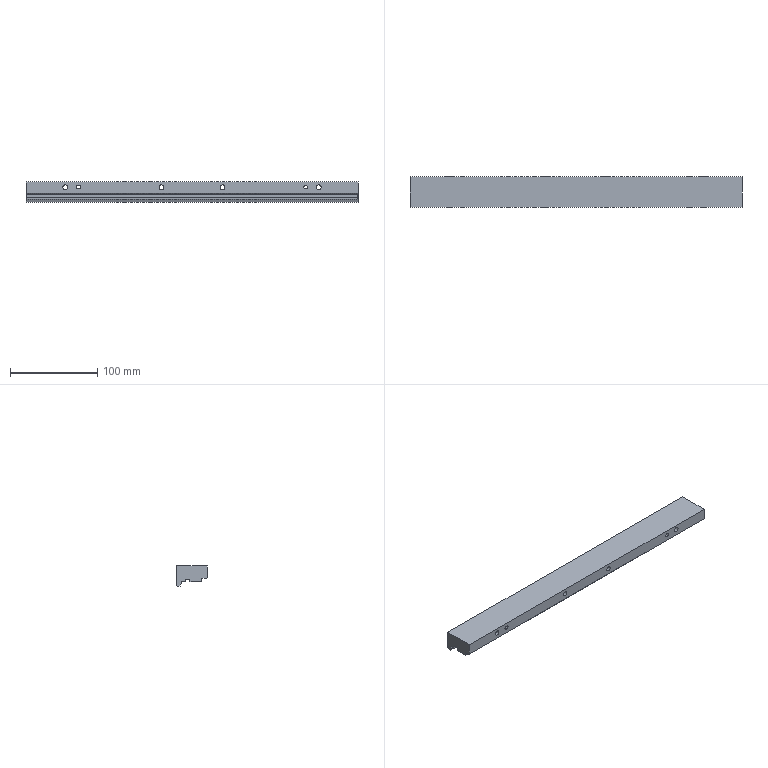Part | NX | 1 solid | 35 faces | box 380 x 35 x 22.9 mm | volume 225857 mm3 | plane 24 | cylinder 11 | commonest cylinder face diameters 5.5 x4 10 x4 4 x3
STEP:
#1=CARTESIAN_POINT('',(190.,-17.5,-13.1));
#2=VERTEX_POINT('',#1);
#3=CARTESIAN_POINT('',(190.,-16.5,-14.1));
#4=VERTEX_POINT('',#3);
#5=CARTESIAN_POINT('',(190.,-17.5,-13.1));
#6=DIRECTION('',(0.,0.7071,-0.7071));
#7=VECTOR('',#6,1000.);
#8=LINE('',#5,#7);
#9=EDGE_CURVE('',#2,#4,#8,.T.);
#10=ORIENTED_EDGE('',*,*,#9,.T.);
#11=CARTESIAN_POINT('',(190.,-11.14,-14.1));
#12=VERTEX_POINT('',#11);
#13=CARTESIAN_POINT('',(190.,-17.5,-14.1));
#14=DIRECTION('',(0.,-1.,0.));
#15=VECTOR('',#14,1000.);
#16=LINE('',#13,#15);
#17=EDGE_CURVE('',#12,#4,#16,.T.);
#18=ORIENTED_EDGE('',*,*,#17,.F.);
#19=CARTESIAN_POINT('',(190.,-11.14,-17.9));
#20=VERTEX_POINT('',#19);
#21=CARTESIAN_POINT('',(190.,-11.14,-14.1));
#22=DIRECTION('',(0.,0.,1.));
#23=VECTOR('',#22,1000.);
#24=LINE('',#21,#23);
#25=EDGE_CURVE('',#20,#12,#24,.T.);
#26=ORIENTED_EDGE('',*,*,#25,.F.);
#27=CARTESIAN_POINT('',(190.,2.3,-17.9));
#28=VERTEX_POINT('',#27);
#29=CARTESIAN_POINT('',(190.,17.5,-17.9));
#30=DIRECTION('',(0.,-1.,0.));
#31=VECTOR('',#30,1000.);
#32=LINE('',#29,#31);
#33=EDGE_CURVE('',#28,#20,#32,.T.);
#34=ORIENTED_EDGE('',*,*,#33,.F.);
#35=CARTESIAN_POINT('',(190.,2.3,-14.9));
#36=VERTEX_POINT('',#35);
#37=CARTESIAN_POINT('',(190.,2.3,-17.9));
#38=DIRECTION('',(0.,0.,-1.));
#39=VECTOR('',#38,1000.);
#40=LINE('',#37,#39);
#41=EDGE_CURVE('',#36,#28,#40,.T.);
#42=ORIENTED_EDGE('',*,*,#41,.F.);
#43=CARTESIAN_POINT('',(190.,7.3,-14.9));
#44=VERTEX_POINT('',#43);
#45=CARTESIAN_POINT('',(190.,2.3,-14.9));
#46=DIRECTION('',(0.,-1.,0.));
#47=VECTOR('',#46,1000.);
#48=LINE('',#45,#47);
#49=EDGE_CURVE('',#44,#36,#48,.T.);
#50=ORIENTED_EDGE('',*,*,#49,.F.);
#51=CARTESIAN_POINT('',(190.,7.3,-17.04));
#52=VERTEX_POINT('',#51);
#53=CARTESIAN_POINT('',(190.,7.3,-14.9));
#54=DIRECTION('',(0.,0.,1.));
#55=VECTOR('',#54,1000.);
#56=LINE('',#53,#55);
#57=EDGE_CURVE('',#52,#44,#56,.T.);
#58=ORIENTED_EDGE('',*,*,#57,.F.);
#59=CARTESIAN_POINT('',(190.,7.533,-17.54));
#60=VERTEX_POINT('',#59);
#61=CARTESIAN_POINT('',(190.,7.3,-17.04));
#62=DIRECTION('',(0.,0.4226,-0.9063));
#63=VECTOR('',#62,1000.);
#64=LINE('',#61,#63);
#65=EDGE_CURVE('',#52,#60,#64,.T.);
#66=ORIENTED_EDGE('',*,*,#65,.T.);
#67=CARTESIAN_POINT('',(190.,12.2,-17.54));
#68=VERTEX_POINT('',#67);
#69=CARTESIAN_POINT('',(190.,7.3,-17.54));
#70=DIRECTION('',(0.,-1.,0.));
#71=VECTOR('',#70,1000.);
#72=LINE('',#69,#71);
#73=EDGE_CURVE('',#68,#60,#72,.T.);
#74=ORIENTED_EDGE('',*,*,#73,.F.);
#75=CARTESIAN_POINT('',(190.,12.2,-19.9));
#76=VERTEX_POINT('',#75);
#77=CARTESIAN_POINT('',(190.,12.2,-17.54));
#78=DIRECTION('',(0.,0.,1.));
#79=VECTOR('',#78,1000.);
#80=LINE('',#77,#79);
#81=EDGE_CURVE('',#76,#68,#80,.T.);
#82=ORIENTED_EDGE('',*,*,#81,.F.);
#83=CARTESIAN_POINT('',(190.,13.599,-22.9));
#84=VERTEX_POINT('',#83);
#85=CARTESIAN_POINT('',(190.,13.599,-22.9));
#86=DIRECTION('',(0.,0.4226,-0.9063));
#87=VECTOR('',#86,1000.);
#88=LINE('',#85,#87);
#89=EDGE_CURVE('',#76,#84,#88,.T.);
#90=ORIENTED_EDGE('',*,*,#89,.T.);
#91=CARTESIAN_POINT('',(190.,16.5,-22.9));
#92=VERTEX_POINT('',#91);
#93=CARTESIAN_POINT('',(190.,0.,-22.9));
#94=DIRECTION('',(0.,1.,0.));
#95=VECTOR('',#94,1000.);
#96=LINE('',#93,#95);
#97=EDGE_CURVE('',#84,#92,#96,.T.);
#98=ORIENTED_EDGE('',*,*,#97,.T.);
#99=CARTESIAN_POINT('',(190.,17.5,-21.9));
#100=VERTEX_POINT('',#99);
#101=CARTESIAN_POINT('',(190.,16.5,-22.9));
#102=DIRECTION('',(0.,0.7071,0.7071));
#103=VECTOR('',#102,1000.);
#104=LINE('',#101,#103);
#105=EDGE_CURVE('',#92,#100,#104,.T.);
#106=ORIENTED_EDGE('',*,*,#105,.T.);
#107=CARTESIAN_POINT('',(190.,17.5,0.));
#108=VERTEX_POINT('',#107);
#109=CARTESIAN_POINT('',(190.,17.5,-17.9));
#110=DIRECTION('',(0.,0.,1.));
#111=VECTOR('',#110,1000.);
#112=LINE('',#109,#111);
#113=EDGE_CURVE('',#100,#108,#112,.T.);
#114=ORIENTED_EDGE('',*,*,#113,.T.);
#115=CARTESIAN_POINT('',(190.,-17.5,0.));
#116=VERTEX_POINT('',#115);
#117=CARTESIAN_POINT('',(190.,17.5,0.));
#118=DIRECTION('',(0.,1.,0.));
#119=VECTOR('',#118,1000.);
#120=LINE('',#117,#119);
#121=EDGE_CURVE('',#116,#108,#120,.T.);
#122=ORIENTED_EDGE('',*,*,#121,.F.);
#123=CARTESIAN_POINT('',(190.,-17.5,-17.9));
#124=DIRECTION('',(0.,0.,1.));
#125=VECTOR('',#124,1000.);
#126=LINE('',#123,#125);
#127=EDGE_CURVE('',#2,#116,#126,.T.);
#128=ORIENTED_EDGE('',*,*,#127,.F.);
#129=EDGE_LOOP('',(#10,#18,#26,#34,#42,#50,#58,#66,#74,#82,#90,#98,#106,#114,#122,#128));
#130=FACE_BOUND('',#129,.T.);
#131=CARTESIAN_POINT('',(190.,17.5,-22.91));
#132=DIRECTION('',(-1.,0.,0.));
#133=DIRECTION('',(0.,0.,-1.));
#134=AXIS2_PLACEMENT_3D('',#131,#132,#133);
#135=PLANE('',#134);
#136=ADVANCED_FACE('',(#130),#135,.F.);
#137=CARTESIAN_POINT('',(-190.,-17.5,-13.1));
#138=VERTEX_POINT('',#137);
#139=CARTESIAN_POINT('',(-190.,-16.5,-14.1));
#140=VERTEX_POINT('',#139);
#141=CARTESIAN_POINT('',(-190.,-17.5,-13.1));
#142=DIRECTION('',(0.,0.7071,-0.7071));
#143=VECTOR('',#142,1000.);
#144=LINE('',#141,#143);
#145=EDGE_CURVE('',#138,#140,#144,.T.);
#146=ORIENTED_EDGE('',*,*,#145,.F.);
#147=CARTESIAN_POINT('',(-190.,-17.5,0.));
#148=VERTEX_POINT('',#147);
#149=CARTESIAN_POINT('',(-190.,-17.5,-17.9));
#150=DIRECTION('',(0.,0.,1.));
#151=VECTOR('',#150,1000.);
#152=LINE('',#149,#151);
#153=EDGE_CURVE('',#138,#148,#152,.T.);
#154=ORIENTED_EDGE('',*,*,#153,.T.);
#155=CARTESIAN_POINT('',(-190.,17.5,0.));
#156=VERTEX_POINT('',#155);
#157=CARTESIAN_POINT('',(-190.,17.5,0.));
#158=DIRECTION('',(0.,1.,0.));
#159=VECTOR('',#158,1000.);
#160=LINE('',#157,#159);
#161=EDGE_CURVE('',#148,#156,#160,.T.);
#162=ORIENTED_EDGE('',*,*,#161,.T.);
#163=CARTESIAN_POINT('',(-190.,17.5,-21.9));
#164=VERTEX_POINT('',#163);
#165=CARTESIAN_POINT('',(-190.,17.5,-17.9));
#166=DIRECTION('',(0.,0.,1.));
#167=VECTOR('',#166,1000.);
#168=LINE('',#165,#167);
#169=EDGE_CURVE('',#164,#156,#168,.T.);
#170=ORIENTED_EDGE('',*,*,#169,.F.);
#171=CARTESIAN_POINT('',(-190.,16.5,-22.9));
#172=VERTEX_POINT('',#171);
#173=CARTESIAN_POINT('',(-190.,16.5,-22.9));
#174=DIRECTION('',(0.,0.7071,0.7071));
#175=VECTOR('',#174,1000.);
#176=LINE('',#173,#175);
#177=EDGE_CURVE('',#172,#164,#176,.T.);
#178=ORIENTED_EDGE('',*,*,#177,.F.);
#179=CARTESIAN_POINT('',(-190.,13.599,-22.9));
#180=VERTEX_POINT('',#179);
#181=CARTESIAN_POINT('',(-190.,0.,-22.9));
#182=DIRECTION('',(0.,1.,0.));
#183=VECTOR('',#182,1000.);
#184=LINE('',#181,#183);
#185=EDGE_CURVE('',#180,#172,#184,.T.);
#186=ORIENTED_EDGE('',*,*,#185,.F.);
#187=CARTESIAN_POINT('',(-190.,12.2,-19.9));
#188=VERTEX_POINT('',#187);
#189=CARTESIAN_POINT('',(-190.,13.599,-22.9));
#190=DIRECTION('',(0.,0.4226,-0.9063));
#191=VECTOR('',#190,1000.);
#192=LINE('',#189,#191);
#193=EDGE_CURVE('',#188,#180,#192,.T.);
#194=ORIENTED_EDGE('',*,*,#193,.F.);
#195=CARTESIAN_POINT('',(-190.,12.2,-17.54));
#196=VERTEX_POINT('',#195);
#197=CARTESIAN_POINT('',(-190.,12.2,-17.54));
#198=DIRECTION('',(0.,0.,1.));
#199=VECTOR('',#198,1000.);
#200=LINE('',#197,#199);
#201=EDGE_CURVE('',#188,#196,#200,.T.);
#202=ORIENTED_EDGE('',*,*,#201,.T.);
#203=CARTESIAN_POINT('',(-190.,7.533,-17.54));
#204=VERTEX_POINT('',#203);
#205=CARTESIAN_POINT('',(-190.,7.3,-17.54));
#206=DIRECTION('',(0.,-1.,0.));
#207=VECTOR('',#206,1000.);
#208=LINE('',#205,#207);
#209=EDGE_CURVE('',#196,#204,#208,.T.);
#210=ORIENTED_EDGE('',*,*,#209,.T.);
#211=CARTESIAN_POINT('',(-190.,7.3,-17.04));
#212=VERTEX_POINT('',#211);
#213=CARTESIAN_POINT('',(-190.,7.3,-17.04));
#214=DIRECTION('',(0.,0.4226,-0.9063));
#215=VECTOR('',#214,1000.);
#216=LINE('',#213,#215);
#217=EDGE_CURVE('',#212,#204,#216,.T.);
#218=ORIENTED_EDGE('',*,*,#217,.F.);
#219=CARTESIAN_POINT('',(-190.,7.3,-14.9));
#220=VERTEX_POINT('',#219);
#221=CARTESIAN_POINT('',(-190.,7.3,-14.9));
#222=DIRECTION('',(0.,0.,1.));
#223=VECTOR('',#222,1000.);
#224=LINE('',#221,#223);
#225=EDGE_CURVE('',#212,#220,#224,.T.);
#226=ORIENTED_EDGE('',*,*,#225,.T.);
#227=CARTESIAN_POINT('',(-190.,2.3,-14.9));
#228=VERTEX_POINT('',#227);
#229=CARTESIAN_POINT('',(-190.,2.3,-14.9));
#230=DIRECTION('',(0.,-1.,0.));
#231=VECTOR('',#230,1000.);
#232=LINE('',#229,#231);
#233=EDGE_CURVE('',#220,#228,#232,.T.);
#234=ORIENTED_EDGE('',*,*,#233,.T.);
#235=CARTESIAN_POINT('',(-190.,2.3,-17.9));
#236=VERTEX_POINT('',#235);
#237=CARTESIAN_POINT('',(-190.,2.3,-17.9));
#238=DIRECTION('',(0.,0.,-1.));
#239=VECTOR('',#238,1000.);
#240=LINE('',#237,#239);
#241=EDGE_CURVE('',#228,#236,#240,.T.);
#242=ORIENTED_EDGE('',*,*,#241,.T.);
#243=CARTESIAN_POINT('',(-190.,-11.14,-17.9));
#244=VERTEX_POINT('',#243);
#245=CARTESIAN_POINT('',(-190.,17.5,-17.9));
#246=DIRECTION('',(0.,-1.,0.));
#247=VECTOR('',#246,1000.);
#248=LINE('',#245,#247);
#249=EDGE_CURVE('',#236,#244,#248,.T.);
#250=ORIENTED_EDGE('',*,*,#249,.T.);
#251=CARTESIAN_POINT('',(-190.,-11.14,-14.1));
#252=VERTEX_POINT('',#251);
#253=CARTESIAN_POINT('',(-190.,-11.14,-14.1));
#254=DIRECTION('',(0.,0.,1.));
#255=VECTOR('',#254,1000.);
#256=LINE('',#253,#255);
#257=EDGE_CURVE('',#244,#252,#256,.T.);
#258=ORIENTED_EDGE('',*,*,#257,.T.);
#259=CARTESIAN_POINT('',(-190.,-17.5,-14.1));
#260=DIRECTION('',(0.,-1.,0.));
#261=VECTOR('',#260,1000.);
#262=LINE('',#259,#261);
#263=EDGE_CURVE('',#252,#140,#262,.T.);
#264=ORIENTED_EDGE('',*,*,#263,.T.);
#265=EDGE_LOOP('',(#146,#154,#162,#170,#178,#186,#194,#202,#210,#218,#226,#234,#242,#250,#258,#264));
#266=FACE_BOUND('',#265,.T.);
#267=CARTESIAN_POINT('',(-190.,17.5,-22.91));
#268=DIRECTION('',(-1.,0.,0.));
#269=DIRECTION('',(0.,0.,-1.));
#270=AXIS2_PLACEMENT_3D('',#267,#268,#269);
#271=PLANE('',#270);
#272=ADVANCED_FACE('',(#266),#271,.T.);
#273=CARTESIAN_POINT('',(730.,12.2,-19.9));
#274=DIRECTION('',(1.,0.,0.));
#275=VECTOR('',#274,1000.);
#276=LINE('',#273,#275);
#277=EDGE_CURVE('',#188,#76,#276,.T.);
#278=ORIENTED_EDGE('',*,*,#277,.F.);
#279=ORIENTED_EDGE('',*,*,#193,.T.);
#280=CARTESIAN_POINT('',(-855.,13.599,-22.9));
#281=DIRECTION('',(-1.,0.,0.));
#282=VECTOR('',#281,1000.);
#283=LINE('',#280,#282);
#284=EDGE_CURVE('',#84,#180,#283,.T.);
#285=ORIENTED_EDGE('',*,*,#284,.F.);
#286=ORIENTED_EDGE('',*,*,#89,.F.);
#287=EDGE_LOOP('',(#278,#279,#285,#286));
#288=FACE_BOUND('',#287,.T.);
#289=CARTESIAN_POINT('',(-62.5,13.599,-22.9));
#290=DIRECTION('',(0.,-0.9063,-0.4226));
#291=DIRECTION('',(-1.,0.,0.));
#292=AXIS2_PLACEMENT_3D('',#289,#290,#291);
#293=PLANE('',#292);
#294=ADVANCED_FACE('',(#288),#293,.T.);
#295=ORIENTED_EDGE('',*,*,#201,.F.);
#296=ORIENTED_EDGE('',*,*,#277,.T.);
#297=ORIENTED_EDGE('',*,*,#81,.T.);
#298=CARTESIAN_POINT('',(-855.,12.2,-17.54));
#299=DIRECTION('',(1.,0.,0.));
#300=VECTOR('',#299,1000.);
#301=LINE('',#298,#300);
#302=EDGE_CURVE('',#196,#68,#301,.T.);
#303=ORIENTED_EDGE('',*,*,#302,.F.);
#304=EDGE_LOOP('',(#295,#296,#297,#303));
#305=FACE_BOUND('',#304,.T.);
#306=CARTESIAN_POINT('',(-855.,12.2,-17.54));
#307=DIRECTION('',(0.,1.,0.));
#308=DIRECTION('',(0.,0.,1.));
#309=AXIS2_PLACEMENT_3D('',#306,#307,#308);
#310=PLANE('',#309);
#311=ADVANCED_FACE('',(#305),#310,.F.);
#312=CARTESIAN_POINT('',(-62.5,16.5,-22.9));
#313=DIRECTION('',(1.,0.,0.));
#314=VECTOR('',#313,1000.);
#315=LINE('',#312,#314);
#316=EDGE_CURVE('',#172,#92,#315,.T.);
#317=ORIENTED_EDGE('',*,*,#316,.F.);
#318=ORIENTED_EDGE('',*,*,#177,.T.);
#319=CARTESIAN_POINT('',(730.,17.5,-21.9));
#320=DIRECTION('',(-1.,0.,0.));
#321=VECTOR('',#320,1000.);
#322=LINE('',#319,#321);
#323=EDGE_CURVE('',#100,#164,#322,.T.);
#324=ORIENTED_EDGE('',*,*,#323,.F.);
#325=ORIENTED_EDGE('',*,*,#105,.F.);
#326=EDGE_LOOP('',(#317,#318,#324,#325));
#327=FACE_BOUND('',#326,.T.);
#328=CARTESIAN_POINT('',(-62.5,16.5,-22.9));
#329=DIRECTION('',(0.,-0.7071,0.7071));
#330=DIRECTION('',(-1.,0.,0.));
#331=AXIS2_PLACEMENT_3D('',#328,#329,#330);
#332=PLANE('',#331);
#333=ADVANCED_FACE('',(#327),#332,.F.);
#334=ORIENTED_EDGE('',*,*,#284,.T.);
#335=ORIENTED_EDGE('',*,*,#185,.T.);
#336=ORIENTED_EDGE('',*,*,#316,.T.);
#337=ORIENTED_EDGE('',*,*,#97,.F.);
#338=EDGE_LOOP('',(#334,#335,#336,#337));
#339=FACE_BOUND('',#338,.T.);
#340=CARTESIAN_POINT('',(-62.5,0.,-22.9));
#341=DIRECTION('',(0.,0.,-1.));
#342=DIRECTION('',(1.,0.,0.));
#343=AXIS2_PLACEMENT_3D('',#340,#341,#342);
#344=PLANE('',#343);
#345=ADVANCED_FACE('',(#339),#344,.T.);
#346=CARTESIAN_POINT('',(-130.5,17.5,-8.));
#347=VERTEX_POINT('',#346);
#348=CARTESIAN_POINT('',(-130.5,17.5,-4.));
#349=VERTEX_POINT('',#348);
#350=CARTESIAN_POINT('',(-130.5,17.5,-6.));
#351=DIRECTION('',(0.,1.,0.));
#352=DIRECTION('',(0.,0.,-1.));
#353=AXIS2_PLACEMENT_3D('',#350,#351,#352);
#354=CIRCLE('',#353,2.);
#355=EDGE_CURVE('',#347,#349,#354,.T.);
#356=ORIENTED_EDGE('',*,*,#355,.F.);
#357=CARTESIAN_POINT('',(-129.5,17.5,-8.));
#358=VERTEX_POINT('',#357);
#359=CARTESIAN_POINT('',(-130.5,17.5,-8.));
#360=DIRECTION('',(-1.,0.,0.));
#361=VECTOR('',#360,1000.);
#362=LINE('',#359,#361);
#363=EDGE_CURVE('',#358,#347,#362,.T.);
#364=ORIENTED_EDGE('',*,*,#363,.F.);
#365=CARTESIAN_POINT('',(-129.5,17.5,-4.));
#366=VERTEX_POINT('',#365);
#367=CARTESIAN_POINT('',(-129.5,17.5,-6.));
#368=DIRECTION('',(0.,1.,0.));
#369=DIRECTION('',(0.,0.,-1.));
#370=AXIS2_PLACEMENT_3D('',#367,#368,#369);
#371=CIRCLE('',#370,2.);
#372=EDGE_CURVE('',#366,#358,#371,.T.);
#373=ORIENTED_EDGE('',*,*,#372,.F.);
#374=CARTESIAN_POINT('',(-130.5,17.5,-4.));
#375=DIRECTION('',(1.,0.,0.));
#376=VECTOR('',#375,1000.);
#377=LINE('',#374,#376);
#378=EDGE_CURVE('',#349,#366,#377,.T.);
#379=ORIENTED_EDGE('',*,*,#378,.F.);
#380=EDGE_LOOP('',(#356,#364,#373,#379));
#381=FACE_BOUND('',#380,.T.);
#382=CARTESIAN_POINT('',(130.,17.5,-8.));
#383=VERTEX_POINT('',#382);
#384=CARTESIAN_POINT('',(130.,17.5,-6.));
#385=DIRECTION('',(0.,1.,0.));
#386=DIRECTION('',(0.,0.,-1.));
#387=AXIS2_PLACEMENT_3D('',#384,#385,#386);
#388=CIRCLE('',#387,2.);
#389=EDGE_CURVE('',#383,#383,#388,.T.);
#390=ORIENTED_EDGE('',*,*,#389,.F.);
#391=EDGE_LOOP('',(#390));
#392=FACE_BOUND('',#391,.T.);
#393=CARTESIAN_POINT('',(145.,17.5,-11.));
#394=VERTEX_POINT('',#393);
#395=CARTESIAN_POINT('',(145.,17.5,-6.));
#396=DIRECTION('',(0.,1.,0.));
#397=DIRECTION('',(0.,0.,-1.));
#398=AXIS2_PLACEMENT_3D('',#395,#396,#397);
#399=CIRCLE('',#398,5.);
#400=EDGE_CURVE('',#394,#394,#399,.T.);
#401=ORIENTED_EDGE('',*,*,#400,.F.);
#402=EDGE_LOOP('',(#401));
#403=FACE_BOUND('',#402,.T.);
#404=CARTESIAN_POINT('',(35.,17.5,-11.));
#405=VERTEX_POINT('',#404);
#406=CARTESIAN_POINT('',(35.,17.5,-6.));
#407=DIRECTION('',(0.,1.,0.));
#408=DIRECTION('',(0.,0.,-1.));
#409=AXIS2_PLACEMENT_3D('',#406,#407,#408);
#410=CIRCLE('',#409,5.);
#411=EDGE_CURVE('',#405,#405,#410,.T.);
#412=ORIENTED_EDGE('',*,*,#411,.F.);
#413=EDGE_LOOP('',(#412));
#414=FACE_BOUND('',#413,.T.);
#415=CARTESIAN_POINT('',(-35.,17.5,-11.));
#416=VERTEX_POINT('',#415);
#417=CARTESIAN_POINT('',(-35.,17.5,-6.));
#418=DIRECTION('',(0.,1.,0.));
#419=DIRECTION('',(0.,0.,-1.));
#420=AXIS2_PLACEMENT_3D('',#417,#418,#419);
#421=CIRCLE('',#420,5.);
#422=EDGE_CURVE('',#416,#416,#421,.T.);
#423=ORIENTED_EDGE('',*,*,#422,.F.);
#424=EDGE_LOOP('',(#423));
#425=FACE_BOUND('',#424,.T.);
#426=CARTESIAN_POINT('',(-145.,17.5,-11.));
#427=VERTEX_POINT('',#426);
#428=CARTESIAN_POINT('',(-145.,17.5,-6.));
#429=DIRECTION('',(0.,1.,0.));
#430=DIRECTION('',(0.,0.,-1.));
#431=AXIS2_PLACEMENT_3D('',#428,#429,#430);
#432=CIRCLE('',#431,5.);
#433=EDGE_CURVE('',#427,#427,#432,.T.);
#434=ORIENTED_EDGE('',*,*,#433,.F.);
#435=EDGE_LOOP('',(#434));
#436=FACE_BOUND('',#435,.T.);
#437=ORIENTED_EDGE('',*,*,#323,.T.);
#438=ORIENTED_EDGE('',*,*,#169,.T.);
#439=CARTESIAN_POINT('',(730.,17.5,0.));
#440=DIRECTION('',(1.,0.,0.));
#441=VECTOR('',#440,1000.);
#442=LINE('',#439,#441);
#443=EDGE_CURVE('',#156,#108,#442,.T.);
#444=ORIENTED_EDGE('',*,*,#443,.T.);
#445=ORIENTED_EDGE('',*,*,#113,.F.);
#446=EDGE_LOOP('',(#437,#438,#444,#445));
#447=FACE_BOUND('',#446,.T.);
#448=CARTESIAN_POINT('',(730.,17.5,-17.9));
#449=DIRECTION('',(0.,1.,0.));
#450=DIRECTION('',(0.,0.,1.));
#451=AXIS2_PLACEMENT_3D('',#448,#449,#450);
#452=PLANE('',#451);
#453=ADVANCED_FACE('',(#381,#392,#403,#414,#425,#436,#447),#452,.T.);
#454=CARTESIAN_POINT('',(-855.,7.3,-17.04));
#455=DIRECTION('',(1.,0.,0.));
#456=VECTOR('',#455,1000.);
#457=LINE('',#454,#456);
#458=EDGE_CURVE('',#212,#52,#457,.T.);
#459=ORIENTED_EDGE('',*,*,#458,.F.);
#460=ORIENTED_EDGE('',*,*,#217,.T.);
#461=CARTESIAN_POINT('',(-855.,7.533,-17.54));
#462=DIRECTION('',(-1.,0.,0.));
#463=VECTOR('',#462,1000.);
#464=LINE('',#461,#463);
#465=EDGE_CURVE('',#60,#204,#464,.T.);
#466=ORIENTED_EDGE('',*,*,#465,.F.);
#467=ORIENTED_EDGE('',*,*,#65,.F.);
#468=EDGE_LOOP('',(#459,#460,#466,#467));
#469=FACE_BOUND('',#468,.T.);
#470=CARTESIAN_POINT('',(-855.,7.3,-17.04));
#471=DIRECTION('',(0.,0.9063,0.4226));
#472=DIRECTION('',(-1.,0.,0.));
#473=AXIS2_PLACEMENT_3D('',#470,#471,#472);
#474=PLANE('',#473);
#475=ADVANCED_FACE('',(#469),#474,.F.);
#476=ORIENTED_EDGE('',*,*,#225,.F.);
#477=ORIENTED_EDGE('',*,*,#458,.T.);
#478=ORIENTED_EDGE('',*,*,#57,.T.);
#479=CARTESIAN_POINT('',(-855.,7.3,-14.9));
#480=DIRECTION('',(1.,0.,0.));
#481=VECTOR('',#480,1000.);
#482=LINE('',#479,#481);
#483=EDGE_CURVE('',#220,#44,#482,.T.);
#484=ORIENTED_EDGE('',*,*,#483,.F.);
#485=EDGE_LOOP('',(#476,#477,#478,#484));
#486=FACE_BOUND('',#485,.T.);
#487=CARTESIAN_POINT('',(-855.,7.3,-14.9));
#488=DIRECTION('',(0.,1.,0.));
#489=DIRECTION('',(0.,0.,1.));
#490=AXIS2_PLACEMENT_3D('',#487,#488,#489);
#491=PLANE('',#490);
#492=ADVANCED_FACE('',(#486),#491,.F.);
#493=ORIENTED_EDGE('',*,*,#209,.F.);
#494=ORIENTED_EDGE('',*,*,#302,.T.);
#495=ORIENTED_EDGE('',*,*,#73,.T.);
#496=ORIENTED_EDGE('',*,*,#465,.T.);
#497=EDGE_LOOP('',(#493,#494,#495,#496));
#498=FACE_BOUND('',#497,.T.);
#499=CARTESIAN_POINT('',(-855.,7.3,-17.54));
#500=DIRECTION('',(0.,0.,1.));
#501=DIRECTION('',(-1.,0.,0.));
#502=AXIS2_PLACEMENT_3D('',#499,#500,#501);
#503=PLANE('',#502);
#504=ADVANCED_FACE('',(#498),#503,.F.);
#505=ORIENTED_EDGE('',*,*,#233,.F.);
#506=ORIENTED_EDGE('',*,*,#483,.T.);
#507=ORIENTED_EDGE('',*,*,#49,.T.);
#508=CARTESIAN_POINT('',(-855.,2.3,-14.9));
#509=DIRECTION('',(1.,0.,0.));
#510=VECTOR('',#509,1000.);
#511=LINE('',#508,#510);
#512=EDGE_CURVE('',#228,#36,#511,.T.);
#513=ORIENTED_EDGE('',*,*,#512,.F.);
#514=EDGE_LOOP('',(#505,#506,#507,#513));
#515=FACE_BOUND('',#514,.T.);
#516=CARTESIAN_POINT('',(-855.,2.3,-14.9));
#517=DIRECTION('',(0.,0.,1.));
#518=DIRECTION('',(-1.,0.,0.));
#519=AXIS2_PLACEMENT_3D('',#516,#517,#518);
#520=PLANE('',#519);
#521=ADVANCED_FACE('',(#515),#520,.F.);
#522=ORIENTED_EDGE('',*,*,#241,.F.);
#523=ORIENTED_EDGE('',*,*,#512,.T.);
#524=ORIENTED_EDGE('',*,*,#41,.T.);
#525=CARTESIAN_POINT('',(-855.,2.3,-17.9));
#526=DIRECTION('',(1.,0.,0.));
#527=VECTOR('',#526,1000.);
#528=LINE('',#525,#527);
#529=EDGE_CURVE('',#236,#28,#528,.T.);
#530=ORIENTED_EDGE('',*,*,#529,.F.);
#531=EDGE_LOOP('',(#522,#523,#524,#530));
#532=FACE_BOUND('',#531,.T.);
#533=CARTESIAN_POINT('',(-855.,2.3,-17.9));
#534=DIRECTION('',(0.,-1.,0.));
#535=DIRECTION('',(0.,0.,-1.));
#536=AXIS2_PLACEMENT_3D('',#533,#534,#535);
#537=PLANE('',#536);
#538=ADVANCED_FACE('',(#532),#537,.F.);
#539=ORIENTED_EDGE('',*,*,#257,.F.);
#540=CARTESIAN_POINT('',(-855.,-11.14,-17.9));
#541=DIRECTION('',(1.,0.,0.));
#542=VECTOR('',#541,1000.);
#543=LINE('',#540,#542);
#544=EDGE_CURVE('',#244,#20,#543,.T.);
#545=ORIENTED_EDGE('',*,*,#544,.T.);
#546=ORIENTED_EDGE('',*,*,#25,.T.);
#547=CARTESIAN_POINT('',(-855.,-11.14,-14.1));
#548=DIRECTION('',(1.,0.,0.));
#549=VECTOR('',#548,1000.);
#550=LINE('',#547,#549);
#551=EDGE_CURVE('',#252,#12,#550,.T.);
#552=ORIENTED_EDGE('',*,*,#551,.F.);
#553=EDGE_LOOP('',(#539,#545,#546,#552));
#554=FACE_BOUND('',#553,.T.);
#555=CARTESIAN_POINT('',(-855.,-11.14,-14.1));
#556=DIRECTION('',(0.,1.,0.));
#557=DIRECTION('',(0.,0.,1.));
#558=AXIS2_PLACEMENT_3D('',#555,#556,#557);
#559=PLANE('',#558);
#560=ADVANCED_FACE('',(#554),#559,.F.);
#561=ORIENTED_EDGE('',*,*,#249,.F.);
#562=ORIENTED_EDGE('',*,*,#529,.T.);
#563=ORIENTED_EDGE('',*,*,#33,.T.);
#564=ORIENTED_EDGE('',*,*,#544,.F.);
#565=EDGE_LOOP('',(#561,#562,#563,#564));
#566=FACE_BOUND('',#565,.T.);
#567=CARTESIAN_POINT('',(730.,17.5,-17.9));
#568=DIRECTION('',(0.,0.,1.));
#569=DIRECTION('',(-1.,0.,0.));
#570=AXIS2_PLACEMENT_3D('',#567,#568,#569);
#571=PLANE('',#570);
#572=ADVANCED_FACE('',(#566),#571,.F.);
#573=CARTESIAN_POINT('',(730.,-17.5,-13.1));
#574=DIRECTION('',(1.,0.,0.));
#575=VECTOR('',#574,1000.);
#576=LINE('',#573,#575);
#577=EDGE_CURVE('',#138,#2,#576,.T.);
#578=ORIENTED_EDGE('',*,*,#577,.F.);
#579=ORIENTED_EDGE('',*,*,#145,.T.);
#580=CARTESIAN_POINT('',(-855.,-16.5,-14.1));
#581=DIRECTION('',(-1.,0.,0.));
#582=VECTOR('',#581,1000.);
#583=LINE('',#580,#582);
#584=EDGE_CURVE('',#4,#140,#583,.T.);
#585=ORIENTED_EDGE('',*,*,#584,.F.);
#586=ORIENTED_EDGE('',*,*,#9,.F.);
#587=EDGE_LOOP('',(#578,#579,#585,#586));
#588=FACE_BOUND('',#587,.T.);
#589=CARTESIAN_POINT('',(730.,-17.5,-13.1));
#590=DIRECTION('',(0.,0.7071,0.7071));
#591=DIRECTION('',(-1.,0.,0.));
#592=AXIS2_PLACEMENT_3D('',#589,#590,#591);
#593=PLANE('',#592);
#594=ADVANCED_FACE('',(#588),#593,.F.);
#595=CARTESIAN_POINT('',(-129.5,-17.5,-8.));
#596=VERTEX_POINT('',#595);
#597=CARTESIAN_POINT('',(-130.5,-17.5,-8.));
#598=VERTEX_POINT('',#597);
#599=CARTESIAN_POINT('',(-130.5,-17.5,-8.));
#600=DIRECTION('',(-1.,0.,0.));
#601=VECTOR('',#600,1000.);
#602=LINE('',#599,#601);
#603=EDGE_CURVE('',#596,#598,#602,.T.);
#604=ORIENTED_EDGE('',*,*,#603,.T.);
#605=CARTESIAN_POINT('',(-130.5,-17.5,-4.));
#606=VERTEX_POINT('',#605);
#607=CARTESIAN_POINT('',(-130.5,-17.5,-6.));
#608=DIRECTION('',(0.,1.,0.));
#609=DIRECTION('',(0.,0.,-1.));
#610=AXIS2_PLACEMENT_3D('',#607,#608,#609);
#611=CIRCLE('',#610,2.);
#612=EDGE_CURVE('',#598,#606,#611,.T.);
#613=ORIENTED_EDGE('',*,*,#612,.T.);
#614=CARTESIAN_POINT('',(-129.5,-17.5,-4.));
#615=VERTEX_POINT('',#614);
#616=CARTESIAN_POINT('',(-130.5,-17.5,-4.));
#617=DIRECTION('',(1.,0.,0.));
#618=VECTOR('',#617,1000.);
#619=LINE('',#616,#618);
#620=EDGE_CURVE('',#606,#615,#619,.T.);
#621=ORIENTED_EDGE('',*,*,#620,.T.);
#622=CARTESIAN_POINT('',(-129.5,-17.5,-6.));
#623=DIRECTION('',(0.,1.,0.));
#624=DIRECTION('',(0.,0.,-1.));
#625=AXIS2_PLACEMENT_3D('',#622,#623,#624);
#626=CIRCLE('',#625,2.);
#627=EDGE_CURVE('',#615,#596,#626,.T.);
#628=ORIENTED_EDGE('',*,*,#627,.T.);
#629=EDGE_LOOP('',(#604,#613,#621,#628));
#630=FACE_BOUND('',#629,.T.);
#631=CARTESIAN_POINT('',(130.,-17.5,-8.));
#632=VERTEX_POINT('',#631);
#633=CARTESIAN_POINT('',(130.,-17.5,-6.));
#634=DIRECTION('',(0.,1.,0.));
#635=DIRECTION('',(0.,0.,-1.));
#636=AXIS2_PLACEMENT_3D('',#633,#634,#635);
#637=CIRCLE('',#636,2.);
#638=EDGE_CURVE('',#632,#632,#637,.T.);
#639=ORIENTED_EDGE('',*,*,#638,.T.);
#640=EDGE_LOOP('',(#639));
#641=FACE_BOUND('',#640,.T.);
#642=CARTESIAN_POINT('',(145.,-17.5,-8.75));
#643=VERTEX_POINT('',#642);
#644=CARTESIAN_POINT('',(145.,-17.5,-6.));
#645=DIRECTION('',(0.,1.,0.));
#646=DIRECTION('',(0.,0.,-1.));
#647=AXIS2_PLACEMENT_3D('',#644,#645,#646);
#648=CIRCLE('',#647,2.75);
#649=EDGE_CURVE('',#643,#643,#648,.T.);
#650=ORIENTED_EDGE('',*,*,#649,.T.);
#651=EDGE_LOOP('',(#650));
#652=FACE_BOUND('',#651,.T.);
#653=CARTESIAN_POINT('',(35.,-17.5,-8.75));
#654=VERTEX_POINT('',#653);
#655=CARTESIAN_POINT('',(35.,-17.5,-6.));
#656=DIRECTION('',(0.,1.,0.));
#657=DIRECTION('',(0.,0.,-1.));
#658=AXIS2_PLACEMENT_3D('',#655,#656,#657);
#659=CIRCLE('',#658,2.75);
#660=EDGE_CURVE('',#654,#654,#659,.T.);
#661=ORIENTED_EDGE('',*,*,#660,.T.);
#662=EDGE_LOOP('',(#661));
#663=FACE_BOUND('',#662,.T.);
#664=CARTESIAN_POINT('',(-35.,-17.5,-8.75));
#665=VERTEX_POINT('',#664);
#666=CARTESIAN_POINT('',(-35.,-17.5,-6.));
#667=DIRECTION('',(0.,1.,0.));
#668=DIRECTION('',(0.,0.,-1.));
#669=AXIS2_PLACEMENT_3D('',#666,#667,#668);
#670=CIRCLE('',#669,2.75);
#671=EDGE_CURVE('',#665,#665,#670,.T.);
#672=ORIENTED_EDGE('',*,*,#671,.T.);
#673=EDGE_LOOP('',(#672));
#674=FACE_BOUND('',#673,.T.);
#675=CARTESIAN_POINT('',(-145.,-17.5,-8.75));
#676=VERTEX_POINT('',#675);
#677=CARTESIAN_POINT('',(-145.,-17.5,-6.));
#678=DIRECTION('',(0.,1.,0.));
#679=DIRECTION('',(0.,0.,-1.));
#680=AXIS2_PLACEMENT_3D('',#677,#678,#679);
#681=CIRCLE('',#680,2.75);
#682=EDGE_CURVE('',#676,#676,#681,.T.);
#683=ORIENTED_EDGE('',*,*,#682,.T.);
#684=EDGE_LOOP('',(#683));
#685=FACE_BOUND('',#684,.T.);
#686=ORIENTED_EDGE('',*,*,#153,.F.);
#687=ORIENTED_EDGE('',*,*,#577,.T.);
#688=ORIENTED_EDGE('',*,*,#127,.T.);
#689=CARTESIAN_POINT('',(730.,-17.5,0.));
#690=DIRECTION('',(1.,0.,0.));
#691=VECTOR('',#690,1000.);
#692=LINE('',#689,#691);
#693=EDGE_CURVE('',#148,#116,#692,.T.);
#694=ORIENTED_EDGE('',*,*,#693,.F.);
#695=EDGE_LOOP('',(#686,#687,#688,#694));
#696=FACE_BOUND('',#695,.T.);
#697=CARTESIAN_POINT('',(730.,-17.5,-17.9));
#698=DIRECTION('',(0.,1.,0.));
#699=DIRECTION('',(0.,0.,1.));
#700=AXIS2_PLACEMENT_3D('',#697,#698,#699);
#701=PLANE('',#700);
#702=ADVANCED_FACE('',(#630,#641,#652,#663,#674,#685,#696),#701,.F.);
#703=ORIENTED_EDGE('',*,*,#263,.F.);
#704=ORIENTED_EDGE('',*,*,#551,.T.);
#705=ORIENTED_EDGE('',*,*,#17,.T.);
#706=ORIENTED_EDGE('',*,*,#584,.T.);
#707=EDGE_LOOP('',(#703,#704,#705,#706));
#708=FACE_BOUND('',#707,.T.);
#709=CARTESIAN_POINT('',(-855.,-17.5,-14.1));
#710=DIRECTION('',(0.,0.,1.));
#711=DIRECTION('',(-1.,0.,0.));
#712=AXIS2_PLACEMENT_3D('',#709,#710,#711);
#713=PLANE('',#712);
#714=ADVANCED_FACE('',(#708),#713,.F.);
#715=ORIENTED_EDGE('',*,*,#161,.F.);
#716=ORIENTED_EDGE('',*,*,#693,.T.);
#717=ORIENTED_EDGE('',*,*,#121,.T.);
#718=ORIENTED_EDGE('',*,*,#443,.F.);
#719=EDGE_LOOP('',(#715,#716,#717,#718));
#720=FACE_BOUND('',#719,.T.);
#721=CARTESIAN_POINT('',(730.,17.5,0.));
#722=DIRECTION('',(0.,0.,-1.));
#723=DIRECTION('',(1.,0.,0.));
#724=AXIS2_PLACEMENT_3D('',#721,#722,#723);
#725=PLANE('',#724);
#726=ADVANCED_FACE('',(#720),#725,.F.);
#727=ORIENTED_EDGE('',*,*,#682,.F.);
#728=EDGE_LOOP('',(#727));
#729=FACE_BOUND('',#728,.T.);
#730=CARTESIAN_POINT('',(-145.,12.1,-8.75));
#731=VERTEX_POINT('',#730);
#732=CARTESIAN_POINT('',(-145.,12.1,-6.));
#733=DIRECTION('',(0.,1.,0.));
#734=DIRECTION('',(0.,0.,-1.));
#735=AXIS2_PLACEMENT_3D('',#732,#733,#734);
#736=CIRCLE('',#735,2.75);
#737=EDGE_CURVE('',#731,#731,#736,.T.);
#738=ORIENTED_EDGE('',*,*,#737,.T.);
#739=EDGE_LOOP('',(#738));
#740=FACE_BOUND('',#739,.T.);
#741=CARTESIAN_POINT('',(-145.,17.5,-6.));
#742=DIRECTION('',(0.,1.,0.));
#743=DIRECTION('',(0.,0.,1.));
#744=AXIS2_PLACEMENT_3D('',#741,#742,#743);
#745=CYLINDRICAL_SURFACE('',#744,2.75);
#746=ADVANCED_FACE('',(#729,#740),#745,.F.);
#747=ORIENTED_EDGE('',*,*,#737,.F.);
#748=EDGE_LOOP('',(#747));
#749=FACE_BOUND('',#748,.T.);
#750=CARTESIAN_POINT('',(-145.,12.1,-11.));
#751=VERTEX_POINT('',#750);
#752=CARTESIAN_POINT('',(-145.,12.1,-6.));
#753=DIRECTION('',(0.,1.,0.));
#754=DIRECTION('',(0.,0.,-1.));
#755=AXIS2_PLACEMENT_3D('',#752,#753,#754);
#756=CIRCLE('',#755,5.);
#757=EDGE_CURVE('',#751,#751,#756,.T.);
#758=ORIENTED_EDGE('',*,*,#757,.T.);
#759=EDGE_LOOP('',(#758));
#760=FACE_BOUND('',#759,.T.);
#761=CARTESIAN_POINT('',(-147.75,12.1,-6.));
#762=DIRECTION('',(0.,-1.,0.));
#763=DIRECTION('',(0.,0.,-1.));
#764=AXIS2_PLACEMENT_3D('',#761,#762,#763);
#765=PLANE('',#764);
#766=ADVANCED_FACE('',(#749,#760),#765,.F.);
#767=ORIENTED_EDGE('',*,*,#757,.F.);
#768=EDGE_LOOP('',(#767));
#769=FACE_BOUND('',#768,.T.);
#770=ORIENTED_EDGE('',*,*,#433,.T.);
#771=EDGE_LOOP('',(#770));
#772=FACE_BOUND('',#771,.T.);
#773=CARTESIAN_POINT('',(-145.,17.5,-6.));
#774=DIRECTION('',(0.,1.,0.));
#775=DIRECTION('',(0.,0.,1.));
#776=AXIS2_PLACEMENT_3D('',#773,#774,#775);
#777=CYLINDRICAL_SURFACE('',#776,5.);
#778=ADVANCED_FACE('',(#769,#772),#777,.F.);
#779=ORIENTED_EDGE('',*,*,#671,.F.);
#780=EDGE_LOOP('',(#779));
#781=FACE_BOUND('',#780,.T.);
#782=CARTESIAN_POINT('',(-35.,12.1,-8.75));
#783=VERTEX_POINT('',#782);
#784=CARTESIAN_POINT('',(-35.,12.1,-6.));
#785=DIRECTION('',(0.,1.,0.));
#786=DIRECTION('',(0.,0.,-1.));
#787=AXIS2_PLACEMENT_3D('',#784,#785,#786);
#788=CIRCLE('',#787,2.75);
#789=EDGE_CURVE('',#783,#783,#788,.T.);
#790=ORIENTED_EDGE('',*,*,#789,.T.);
#791=EDGE_LOOP('',(#790));
#792=FACE_BOUND('',#791,.T.);
#793=CARTESIAN_POINT('',(-35.,17.5,-6.));
#794=DIRECTION('',(0.,1.,0.));
#795=DIRECTION('',(0.,0.,1.));
#796=AXIS2_PLACEMENT_3D('',#793,#794,#795);
#797=CYLINDRICAL_SURFACE('',#796,2.75);
#798=ADVANCED_FACE('',(#781,#792),#797,.F.);
#799=ORIENTED_EDGE('',*,*,#789,.F.);
#800=EDGE_LOOP('',(#799));
#801=FACE_BOUND('',#800,.T.);
#802=CARTESIAN_POINT('',(-35.,12.1,-11.));
#803=VERTEX_POINT('',#802);
#804=CARTESIAN_POINT('',(-35.,12.1,-6.));
#805=DIRECTION('',(0.,1.,0.));
#806=DIRECTION('',(0.,0.,-1.));
#807=AXIS2_PLACEMENT_3D('',#804,#805,#806);
#808=CIRCLE('',#807,5.);
#809=EDGE_CURVE('',#803,#803,#808,.T.);
#810=ORIENTED_EDGE('',*,*,#809,.T.);
#811=EDGE_LOOP('',(#810));
#812=FACE_BOUND('',#811,.T.);
#813=CARTESIAN_POINT('',(-37.75,12.1,-6.));
#814=DIRECTION('',(0.,-1.,0.));
#815=DIRECTION('',(0.,0.,-1.));
#816=AXIS2_PLACEMENT_3D('',#813,#814,#815);
#817=PLANE('',#816);
#818=ADVANCED_FACE('',(#801,#812),#817,.F.);
#819=ORIENTED_EDGE('',*,*,#809,.F.);
#820=EDGE_LOOP('',(#819));
#821=FACE_BOUND('',#820,.T.);
#822=ORIENTED_EDGE('',*,*,#422,.T.);
#823=EDGE_LOOP('',(#822));
#824=FACE_BOUND('',#823,.T.);
#825=CARTESIAN_POINT('',(-35.,17.5,-6.));
#826=DIRECTION('',(0.,1.,0.));
#827=DIRECTION('',(0.,0.,1.));
#828=AXIS2_PLACEMENT_3D('',#825,#826,#827);
#829=CYLINDRICAL_SURFACE('',#828,5.);
#830=ADVANCED_FACE('',(#821,#824),#829,.F.);
#831=ORIENTED_EDGE('',*,*,#660,.F.);
#832=EDGE_LOOP('',(#831));
#833=FACE_BOUND('',#832,.T.);
#834=CARTESIAN_POINT('',(35.,12.1,-8.75));
#835=VERTEX_POINT('',#834);
#836=CARTESIAN_POINT('',(35.,12.1,-6.));
#837=DIRECTION('',(0.,1.,0.));
#838=DIRECTION('',(0.,0.,-1.));
#839=AXIS2_PLACEMENT_3D('',#836,#837,#838);
#840=CIRCLE('',#839,2.75);
#841=EDGE_CURVE('',#835,#835,#840,.T.);
#842=ORIENTED_EDGE('',*,*,#841,.T.);
#843=EDGE_LOOP('',(#842));
#844=FACE_BOUND('',#843,.T.);
#845=CARTESIAN_POINT('',(35.,17.5,-6.));
#846=DIRECTION('',(0.,1.,0.));
#847=DIRECTION('',(0.,0.,1.));
#848=AXIS2_PLACEMENT_3D('',#845,#846,#847);
#849=CYLINDRICAL_SURFACE('',#848,2.75);
#850=ADVANCED_FACE('',(#833,#844),#849,.F.);
#851=ORIENTED_EDGE('',*,*,#841,.F.);
#852=EDGE_LOOP('',(#851));
#853=FACE_BOUND('',#852,.T.);
#854=CARTESIAN_POINT('',(35.,12.1,-11.));
#855=VERTEX_POINT('',#854);
#856=CARTESIAN_POINT('',(35.,12.1,-6.));
#857=DIRECTION('',(0.,1.,0.));
#858=DIRECTION('',(0.,0.,-1.));
#859=AXIS2_PLACEMENT_3D('',#856,#857,#858);
#860=CIRCLE('',#859,5.);
#861=EDGE_CURVE('',#855,#855,#860,.T.);
#862=ORIENTED_EDGE('',*,*,#861,.T.);
#863=EDGE_LOOP('',(#862));
#864=FACE_BOUND('',#863,.T.);
#865=CARTESIAN_POINT('',(32.25,12.1,-6.));
#866=DIRECTION('',(0.,-1.,0.));
#867=DIRECTION('',(0.,0.,-1.));
#868=AXIS2_PLACEMENT_3D('',#865,#866,#867);
#869=PLANE('',#868);
#870=ADVANCED_FACE('',(#853,#864),#869,.F.);
#871=ORIENTED_EDGE('',*,*,#861,.F.);
#872=EDGE_LOOP('',(#871));
#873=FACE_BOUND('',#872,.T.);
#874=ORIENTED_EDGE('',*,*,#411,.T.);
#875=EDGE_LOOP('',(#874));
#876=FACE_BOUND('',#875,.T.);
#877=CARTESIAN_POINT('',(35.,17.5,-6.));
#878=DIRECTION('',(0.,1.,0.));
#879=DIRECTION('',(0.,0.,1.));
#880=AXIS2_PLACEMENT_3D('',#877,#878,#879);
#881=CYLINDRICAL_SURFACE('',#880,5.);
#882=ADVANCED_FACE('',(#873,#876),#881,.F.);
#883=ORIENTED_EDGE('',*,*,#649,.F.);
#884=EDGE_LOOP('',(#883));
#885=FACE_BOUND('',#884,.T.);
#886=CARTESIAN_POINT('',(145.,12.1,-8.75));
#887=VERTEX_POINT('',#886);
#888=CARTESIAN_POINT('',(145.,12.1,-6.));
#889=DIRECTION('',(0.,1.,0.));
#890=DIRECTION('',(0.,0.,-1.));
#891=AXIS2_PLACEMENT_3D('',#888,#889,#890);
#892=CIRCLE('',#891,2.75);
#893=EDGE_CURVE('',#887,#887,#892,.T.);
#894=ORIENTED_EDGE('',*,*,#893,.T.);
#895=EDGE_LOOP('',(#894));
#896=FACE_BOUND('',#895,.T.);
#897=CARTESIAN_POINT('',(145.,17.5,-6.));
#898=DIRECTION('',(0.,1.,0.));
#899=DIRECTION('',(0.,0.,1.));
#900=AXIS2_PLACEMENT_3D('',#897,#898,#899);
#901=CYLINDRICAL_SURFACE('',#900,2.75);
#902=ADVANCED_FACE('',(#885,#896),#901,.F.);
#903=ORIENTED_EDGE('',*,*,#893,.F.);
#904=EDGE_LOOP('',(#903));
#905=FACE_BOUND('',#904,.T.);
#906=CARTESIAN_POINT('',(145.,12.1,-11.));
#907=VERTEX_POINT('',#906);
#908=CARTESIAN_POINT('',(145.,12.1,-6.));
#909=DIRECTION('',(0.,1.,0.));
#910=DIRECTION('',(0.,0.,-1.));
#911=AXIS2_PLACEMENT_3D('',#908,#909,#910);
#912=CIRCLE('',#911,5.);
#913=EDGE_CURVE('',#907,#907,#912,.T.);
#914=ORIENTED_EDGE('',*,*,#913,.T.);
#915=EDGE_LOOP('',(#914));
#916=FACE_BOUND('',#915,.T.);
#917=CARTESIAN_POINT('',(142.25,12.1,-6.));
#918=DIRECTION('',(0.,-1.,0.));
#919=DIRECTION('',(0.,0.,-1.));
#920=AXIS2_PLACEMENT_3D('',#917,#918,#919);
#921=PLANE('',#920);
#922=ADVANCED_FACE('',(#905,#916),#921,.F.);
#923=ORIENTED_EDGE('',*,*,#913,.F.);
#924=EDGE_LOOP('',(#923));
#925=FACE_BOUND('',#924,.T.);
#926=ORIENTED_EDGE('',*,*,#400,.T.);
#927=EDGE_LOOP('',(#926));
#928=FACE_BOUND('',#927,.T.);
#929=CARTESIAN_POINT('',(145.,17.5,-6.));
#930=DIRECTION('',(0.,1.,0.));
#931=DIRECTION('',(0.,0.,1.));
#932=AXIS2_PLACEMENT_3D('',#929,#930,#931);
#933=CYLINDRICAL_SURFACE('',#932,5.);
#934=ADVANCED_FACE('',(#925,#928),#933,.F.);
#935=ORIENTED_EDGE('',*,*,#638,.F.);
#936=EDGE_LOOP('',(#935));
#937=FACE_BOUND('',#936,.T.);
#938=ORIENTED_EDGE('',*,*,#389,.T.);
#939=EDGE_LOOP('',(#938));
#940=FACE_BOUND('',#939,.T.);
#941=CARTESIAN_POINT('',(130.,-17.5,-6.));
#942=DIRECTION('',(0.,1.,0.));
#943=DIRECTION('',(0.,0.,1.));
#944=AXIS2_PLACEMENT_3D('',#941,#942,#943);
#945=CYLINDRICAL_SURFACE('',#944,2.);
#946=ADVANCED_FACE('',(#937,#940),#945,.F.);
#947=ORIENTED_EDGE('',*,*,#355,.T.);
#948=CARTESIAN_POINT('',(-130.5,-17.5,-4.));
#949=DIRECTION('',(0.,1.,0.));
#950=VECTOR('',#949,1000.);
#951=LINE('',#948,#950);
#952=EDGE_CURVE('',#606,#349,#951,.T.);
#953=ORIENTED_EDGE('',*,*,#952,.F.);
#954=ORIENTED_EDGE('',*,*,#612,.F.);
#955=CARTESIAN_POINT('',(-130.5,-17.5,-8.));
#956=DIRECTION('',(0.,1.,0.));
#957=VECTOR('',#956,1000.);
#958=LINE('',#955,#957);
#959=EDGE_CURVE('',#598,#347,#958,.T.);
#960=ORIENTED_EDGE('',*,*,#959,.T.);
#961=EDGE_LOOP('',(#947,#953,#954,#960));
#962=FACE_BOUND('',#961,.T.);
#963=CARTESIAN_POINT('',(-130.5,-17.5,-6.));
#964=DIRECTION('',(0.,1.,0.));
#965=DIRECTION('',(0.,0.,1.));
#966=AXIS2_PLACEMENT_3D('',#963,#964,#965);
#967=CYLINDRICAL_SURFACE('',#966,2.);
#968=ADVANCED_FACE('',(#962),#967,.F.);
#969=ORIENTED_EDGE('',*,*,#363,.T.);
#970=ORIENTED_EDGE('',*,*,#959,.F.);
#971=ORIENTED_EDGE('',*,*,#603,.F.);
#972=CARTESIAN_POINT('',(-129.5,-17.5,-8.));
#973=DIRECTION('',(0.,1.,0.));
#974=VECTOR('',#973,1000.);
#975=LINE('',#972,#974);
#976=EDGE_CURVE('',#596,#358,#975,.T.);
#977=ORIENTED_EDGE('',*,*,#976,.T.);
#978=EDGE_LOOP('',(#969,#970,#971,#977));
#979=FACE_BOUND('',#978,.T.);
#980=CARTESIAN_POINT('',(-130.5,-17.5,-8.));
#981=DIRECTION('',(0.,0.,-1.));
#982=DIRECTION('',(1.,0.,0.));
#983=AXIS2_PLACEMENT_3D('',#980,#981,#982);
#984=PLANE('',#983);
#985=ADVANCED_FACE('',(#979),#984,.F.);
#986=ORIENTED_EDGE('',*,*,#372,.T.);
#987=ORIENTED_EDGE('',*,*,#976,.F.);
#988=ORIENTED_EDGE('',*,*,#627,.F.);
#989=CARTESIAN_POINT('',(-129.5,-17.5,-4.));
#990=DIRECTION('',(0.,1.,0.));
#991=VECTOR('',#990,1000.);
#992=LINE('',#989,#991);
#993=EDGE_CURVE('',#615,#366,#992,.T.);
#994=ORIENTED_EDGE('',*,*,#993,.T.);
#995=EDGE_LOOP('',(#986,#987,#988,#994));
#996=FACE_BOUND('',#995,.T.);
#997=CARTESIAN_POINT('',(-129.5,-17.5,-6.));
#998=DIRECTION('',(0.,1.,0.));
#999=DIRECTION('',(0.,0.,1.));
#1000=AXIS2_PLACEMENT_3D('',#997,#998,#999);
#1001=CYLINDRICAL_SURFACE('',#1000,2.);
#1002=ADVANCED_FACE('',(#996),#1001,.F.);
#1003=ORIENTED_EDGE('',*,*,#378,.T.);
#1004=ORIENTED_EDGE('',*,*,#993,.F.);
#1005=ORIENTED_EDGE('',*,*,#620,.F.);
#1006=ORIENTED_EDGE('',*,*,#952,.T.);
#1007=EDGE_LOOP('',(#1003,#1004,#1005,#1006));
#1008=FACE_BOUND('',#1007,.T.);
#1009=CARTESIAN_POINT('',(-130.5,-17.5,-4.));
#1010=DIRECTION('',(0.,0.,1.));
#1011=DIRECTION('',(-1.,0.,0.));
#1012=AXIS2_PLACEMENT_3D('',#1009,#1010,#1011);
#1013=PLANE('',#1012);
#1014=ADVANCED_FACE('',(#1008),#1013,.F.);
#1015=CLOSED_SHELL('',(#136,#272,#294,#311,#333,#345,#453,#475,#492,#504,#521,#538,#560,#572,#594,#702,#714,#726,#746,#766,#778,#798,#818,#830,#850,#870,#882,#902,#922,#934,#946,#968,#985,#1002,#1014));
#1016=MANIFOLD_SOLID_BREP('',#1015);
#1017=(LENGTH_UNIT()NAMED_UNIT(*)SI_UNIT(.MILLI.,.METRE.));
#1018=UNCERTAINTY_MEASURE_WITH_UNIT(LENGTH_MEASURE(0.00001),#1017,'','');
#1019=(NAMED_UNIT(*)PLANE_ANGLE_UNIT()SI_UNIT($,.RADIAN.));
#1020=(NAMED_UNIT(*)SI_UNIT($,.STERADIAN.)SOLID_ANGLE_UNIT());
#1021=(GEOMETRIC_REPRESENTATION_CONTEXT(3)GLOBAL_UNCERTAINTY_ASSIGNED_CONTEXT((#1018))GLOBAL_UNIT_ASSIGNED_CONTEXT((#1017,#1019,#1020))REPRESENTATION_CONTEXT('',''));
#1022=ADVANCED_BREP_SHAPE_REPRESENTATION('',(#1016),#1021);